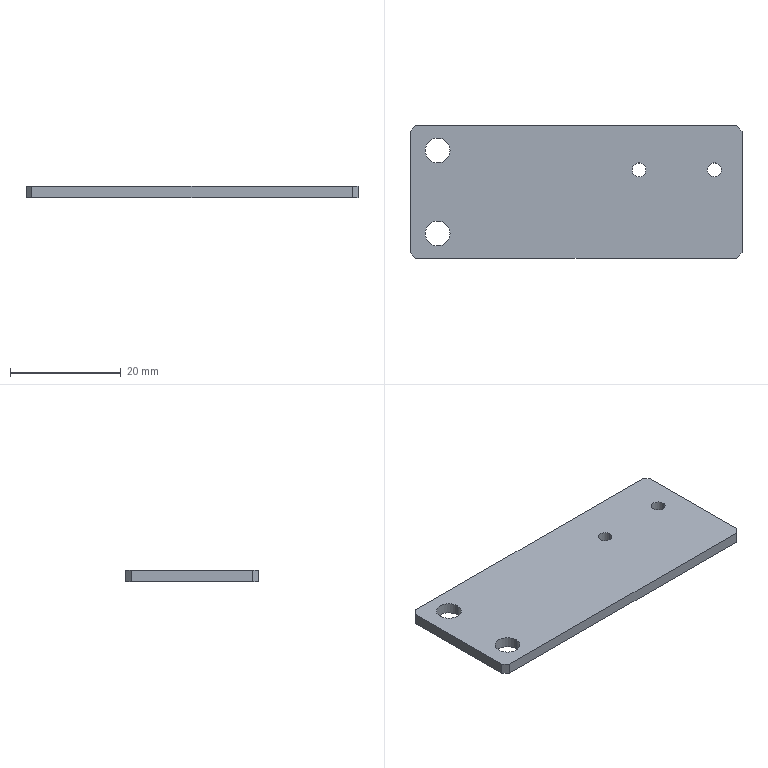Part | SolidWorks | features HoleWzd 2, Chamfer 1, FlatPattern 1, SMBaseFlange 1, SheetMetal 1 | 1 solid | 18 faces | box 60 x 24 x 2 mm | volume 2793 mm3 | plane 10 | cylinder 8 | commonest cylinder face diameters 2.5 x4 4.5 x4
STEP:
#1=CARTESIAN_POINT('',(10.15,4.,-2.));
#2=VERTEX_POINT('',#1);
#3=CARTESIAN_POINT('',(12.65,4.,-2.));
#4=VERTEX_POINT('',#3);
#5=CARTESIAN_POINT('',(11.4,4.,-2.));
#6=DIRECTION('',(0.,0.,1.));
#7=DIRECTION('',(1.,0.,0.));
#8=AXIS2_PLACEMENT_3D('',#5,#6,#7);
#9=CIRCLE('',#8,1.25);
#10=EDGE_CURVE('',#2,#4,#9,.T.);
#11=ORIENTED_EDGE('',*,*,#10,.F.);
#12=CARTESIAN_POINT('',(10.15,4.,0.));
#13=VERTEX_POINT('',#12);
#14=CARTESIAN_POINT('',(10.15,4.,0.));
#15=DIRECTION('',(0.,0.,1.));
#16=VECTOR('',#15,1000.);
#17=LINE('',#14,#16);
#18=EDGE_CURVE('',#2,#13,#17,.T.);
#19=ORIENTED_EDGE('',*,*,#18,.T.);
#20=CARTESIAN_POINT('',(12.65,4.,0.));
#21=VERTEX_POINT('',#20);
#22=CARTESIAN_POINT('',(11.4,4.,0.));
#23=DIRECTION('',(0.,0.,1.));
#24=DIRECTION('',(1.,0.,0.));
#25=AXIS2_PLACEMENT_3D('',#22,#23,#24);
#26=CIRCLE('',#25,1.25);
#27=EDGE_CURVE('',#13,#21,#26,.T.);
#28=ORIENTED_EDGE('',*,*,#27,.T.);
#29=CARTESIAN_POINT('',(12.65,4.,0.));
#30=DIRECTION('',(0.,0.,1.));
#31=VECTOR('',#30,1000.);
#32=LINE('',#29,#31);
#33=EDGE_CURVE('',#4,#21,#32,.T.);
#34=ORIENTED_EDGE('',*,*,#33,.F.);
#35=EDGE_LOOP('',(#11,#19,#28,#34));
#36=FACE_OUTER_BOUND('',#35,.T.);
#37=CARTESIAN_POINT('',(11.4,4.,0.));
#38=DIRECTION('',(0.,0.,1.));
#39=DIRECTION('',(1.,0.,0.));
#40=AXIS2_PLACEMENT_3D('',#37,#38,#39);
#41=CYLINDRICAL_SURFACE('',#40,1.25);
#42=ADVANCED_FACE('',(#36),#41,.F.);
#43=CARTESIAN_POINT('',(23.75,4.,-2.));
#44=VERTEX_POINT('',#43);
#45=CARTESIAN_POINT('',(26.25,4.,-2.));
#46=VERTEX_POINT('',#45);
#47=CARTESIAN_POINT('',(25.,4.,-2.));
#48=DIRECTION('',(0.,0.,1.));
#49=DIRECTION('',(1.,0.,0.));
#50=AXIS2_PLACEMENT_3D('',#47,#48,#49);
#51=CIRCLE('',#50,1.25);
#52=EDGE_CURVE('',#44,#46,#51,.T.);
#53=ORIENTED_EDGE('',*,*,#52,.F.);
#54=CARTESIAN_POINT('',(23.75,4.,0.));
#55=VERTEX_POINT('',#54);
#56=CARTESIAN_POINT('',(23.75,4.,0.));
#57=DIRECTION('',(0.,0.,1.));
#58=VECTOR('',#57,1000.);
#59=LINE('',#56,#58);
#60=EDGE_CURVE('',#44,#55,#59,.T.);
#61=ORIENTED_EDGE('',*,*,#60,.T.);
#62=CARTESIAN_POINT('',(26.25,4.,0.));
#63=VERTEX_POINT('',#62);
#64=CARTESIAN_POINT('',(25.,4.,0.));
#65=DIRECTION('',(0.,0.,1.));
#66=DIRECTION('',(1.,0.,0.));
#67=AXIS2_PLACEMENT_3D('',#64,#65,#66);
#68=CIRCLE('',#67,1.25);
#69=EDGE_CURVE('',#55,#63,#68,.T.);
#70=ORIENTED_EDGE('',*,*,#69,.T.);
#71=CARTESIAN_POINT('',(26.25,4.,0.));
#72=DIRECTION('',(0.,0.,1.));
#73=VECTOR('',#72,1000.);
#74=LINE('',#71,#73);
#75=EDGE_CURVE('',#46,#63,#74,.T.);
#76=ORIENTED_EDGE('',*,*,#75,.F.);
#77=EDGE_LOOP('',(#53,#61,#70,#76));
#78=FACE_OUTER_BOUND('',#77,.T.);
#79=CARTESIAN_POINT('',(25.,4.,0.));
#80=DIRECTION('',(0.,0.,1.));
#81=DIRECTION('',(1.,0.,0.));
#82=AXIS2_PLACEMENT_3D('',#79,#80,#81);
#83=CYLINDRICAL_SURFACE('',#82,1.25);
#84=ADVANCED_FACE('',(#78),#83,.F.);
#85=CARTESIAN_POINT('',(-27.25,7.5,-2.));
#86=VERTEX_POINT('',#85);
#87=CARTESIAN_POINT('',(-22.75,7.5,-2.));
#88=VERTEX_POINT('',#87);
#89=CARTESIAN_POINT('',(-25.,7.5,-2.));
#90=DIRECTION('',(0.,0.,1.));
#91=DIRECTION('',(1.,0.,0.));
#92=AXIS2_PLACEMENT_3D('',#89,#90,#91);
#93=CIRCLE('',#92,2.25);
#94=EDGE_CURVE('',#86,#88,#93,.T.);
#95=ORIENTED_EDGE('',*,*,#94,.F.);
#96=CARTESIAN_POINT('',(-27.25,7.5,0.));
#97=VERTEX_POINT('',#96);
#98=CARTESIAN_POINT('',(-27.25,7.5,0.));
#99=DIRECTION('',(0.,0.,1.));
#100=VECTOR('',#99,1000.);
#101=LINE('',#98,#100);
#102=EDGE_CURVE('',#86,#97,#101,.T.);
#103=ORIENTED_EDGE('',*,*,#102,.T.);
#104=CARTESIAN_POINT('',(-22.75,7.5,0.));
#105=VERTEX_POINT('',#104);
#106=CARTESIAN_POINT('',(-25.,7.5,0.));
#107=DIRECTION('',(0.,0.,1.));
#108=DIRECTION('',(1.,0.,0.));
#109=AXIS2_PLACEMENT_3D('',#106,#107,#108);
#110=CIRCLE('',#109,2.25);
#111=EDGE_CURVE('',#97,#105,#110,.T.);
#112=ORIENTED_EDGE('',*,*,#111,.T.);
#113=CARTESIAN_POINT('',(-22.75,7.5,0.));
#114=DIRECTION('',(0.,0.,1.));
#115=VECTOR('',#114,1000.);
#116=LINE('',#113,#115);
#117=EDGE_CURVE('',#88,#105,#116,.T.);
#118=ORIENTED_EDGE('',*,*,#117,.F.);
#119=EDGE_LOOP('',(#95,#103,#112,#118));
#120=FACE_OUTER_BOUND('',#119,.T.);
#121=CARTESIAN_POINT('',(-25.,7.5,0.));
#122=DIRECTION('',(0.,0.,1.));
#123=DIRECTION('',(1.,0.,0.));
#124=AXIS2_PLACEMENT_3D('',#121,#122,#123);
#125=CYLINDRICAL_SURFACE('',#124,2.25);
#126=ADVANCED_FACE('',(#120),#125,.F.);
#127=CARTESIAN_POINT('',(-27.25,-7.5,-2.));
#128=VERTEX_POINT('',#127);
#129=CARTESIAN_POINT('',(-22.75,-7.5,-2.));
#130=VERTEX_POINT('',#129);
#131=CARTESIAN_POINT('',(-25.,-7.5,-2.));
#132=DIRECTION('',(0.,0.,1.));
#133=DIRECTION('',(1.,0.,0.));
#134=AXIS2_PLACEMENT_3D('',#131,#132,#133);
#135=CIRCLE('',#134,2.25);
#136=EDGE_CURVE('',#128,#130,#135,.T.);
#137=ORIENTED_EDGE('',*,*,#136,.F.);
#138=CARTESIAN_POINT('',(-27.25,-7.5,0.));
#139=VERTEX_POINT('',#138);
#140=CARTESIAN_POINT('',(-27.25,-7.5,0.));
#141=DIRECTION('',(0.,0.,1.));
#142=VECTOR('',#141,1000.);
#143=LINE('',#140,#142);
#144=EDGE_CURVE('',#128,#139,#143,.T.);
#145=ORIENTED_EDGE('',*,*,#144,.T.);
#146=CARTESIAN_POINT('',(-22.75,-7.5,0.));
#147=VERTEX_POINT('',#146);
#148=CARTESIAN_POINT('',(-25.,-7.5,0.));
#149=DIRECTION('',(0.,0.,1.));
#150=DIRECTION('',(1.,0.,0.));
#151=AXIS2_PLACEMENT_3D('',#148,#149,#150);
#152=CIRCLE('',#151,2.25);
#153=EDGE_CURVE('',#139,#147,#152,.T.);
#154=ORIENTED_EDGE('',*,*,#153,.T.);
#155=CARTESIAN_POINT('',(-22.75,-7.5,0.));
#156=DIRECTION('',(0.,0.,1.));
#157=VECTOR('',#156,1000.);
#158=LINE('',#155,#157);
#159=EDGE_CURVE('',#130,#147,#158,.T.);
#160=ORIENTED_EDGE('',*,*,#159,.F.);
#161=EDGE_LOOP('',(#137,#145,#154,#160));
#162=FACE_OUTER_BOUND('',#161,.T.);
#163=CARTESIAN_POINT('',(-25.,-7.5,0.));
#164=DIRECTION('',(0.,0.,1.));
#165=DIRECTION('',(1.,0.,0.));
#166=AXIS2_PLACEMENT_3D('',#163,#164,#165);
#167=CYLINDRICAL_SURFACE('',#166,2.25);
#168=ADVANCED_FACE('',(#162),#167,.F.);
#169=CARTESIAN_POINT('',(30.,-11.,0.));
#170=VERTEX_POINT('',#169);
#171=CARTESIAN_POINT('',(30.,11.,0.));
#172=VERTEX_POINT('',#171);
#173=CARTESIAN_POINT('',(30.,12.,0.));
#174=DIRECTION('',(0.,1.,0.));
#175=VECTOR('',#174,1000.);
#176=LINE('',#173,#175);
#177=EDGE_CURVE('',#170,#172,#176,.T.);
#178=ORIENTED_EDGE('',*,*,#177,.F.);
#179=CARTESIAN_POINT('',(30.,-11.,-2.));
#180=VERTEX_POINT('',#179);
#181=CARTESIAN_POINT('',(30.,-11.,-2.));
#182=DIRECTION('',(0.,0.,-1.));
#183=VECTOR('',#182,1000.);
#184=LINE('',#181,#183);
#185=EDGE_CURVE('',#170,#180,#184,.T.);
#186=ORIENTED_EDGE('',*,*,#185,.T.);
#187=CARTESIAN_POINT('',(30.,11.,-2.));
#188=VERTEX_POINT('',#187);
#189=CARTESIAN_POINT('',(30.,12.,-2.));
#190=DIRECTION('',(0.,1.,0.));
#191=VECTOR('',#190,1000.);
#192=LINE('',#189,#191);
#193=EDGE_CURVE('',#180,#188,#192,.T.);
#194=ORIENTED_EDGE('',*,*,#193,.T.);
#195=CARTESIAN_POINT('',(30.,11.,-2.));
#196=DIRECTION('',(0.,0.,1.));
#197=VECTOR('',#196,1000.);
#198=LINE('',#195,#197);
#199=EDGE_CURVE('',#188,#172,#198,.T.);
#200=ORIENTED_EDGE('',*,*,#199,.T.);
#201=EDGE_LOOP('',(#178,#186,#194,#200));
#202=FACE_OUTER_BOUND('',#201,.T.);
#203=CARTESIAN_POINT('',(30.,12.,-2.));
#204=DIRECTION('',(1.,0.,0.));
#205=DIRECTION('',(0.,1.,0.));
#206=AXIS2_PLACEMENT_3D('',#203,#204,#205);
#207=PLANE('',#206);
#208=ADVANCED_FACE('',(#202),#207,.T.);
#209=CARTESIAN_POINT('',(-29.,-12.,0.));
#210=VERTEX_POINT('',#209);
#211=CARTESIAN_POINT('',(29.,-12.,0.));
#212=VERTEX_POINT('',#211);
#213=CARTESIAN_POINT('',(-30.,-12.,0.));
#214=DIRECTION('',(1.,0.,0.));
#215=VECTOR('',#214,1000.);
#216=LINE('',#213,#215);
#217=EDGE_CURVE('',#210,#212,#216,.T.);
#218=ORIENTED_EDGE('',*,*,#217,.F.);
#219=CARTESIAN_POINT('',(-29.,-12.,-2.));
#220=VERTEX_POINT('',#219);
#221=CARTESIAN_POINT('',(-29.,-12.,-2.));
#222=DIRECTION('',(0.,0.,-1.));
#223=VECTOR('',#222,1000.);
#224=LINE('',#221,#223);
#225=EDGE_CURVE('',#210,#220,#224,.T.);
#226=ORIENTED_EDGE('',*,*,#225,.T.);
#227=CARTESIAN_POINT('',(29.,-12.,-2.));
#228=VERTEX_POINT('',#227);
#229=CARTESIAN_POINT('',(-30.,-12.,-2.));
#230=DIRECTION('',(1.,0.,0.));
#231=VECTOR('',#230,1000.);
#232=LINE('',#229,#231);
#233=EDGE_CURVE('',#220,#228,#232,.T.);
#234=ORIENTED_EDGE('',*,*,#233,.T.);
#235=CARTESIAN_POINT('',(29.,-12.,-2.));
#236=DIRECTION('',(0.,0.,1.));
#237=VECTOR('',#236,1000.);
#238=LINE('',#235,#237);
#239=EDGE_CURVE('',#228,#212,#238,.T.);
#240=ORIENTED_EDGE('',*,*,#239,.T.);
#241=EDGE_LOOP('',(#218,#226,#234,#240));
#242=FACE_OUTER_BOUND('',#241,.T.);
#243=CARTESIAN_POINT('',(-30.,-12.,-2.));
#244=DIRECTION('',(0.,-1.,0.));
#245=DIRECTION('',(0.,0.,-1.));
#246=AXIS2_PLACEMENT_3D('',#243,#244,#245);
#247=PLANE('',#246);
#248=ADVANCED_FACE('',(#242),#247,.T.);
#249=CARTESIAN_POINT('',(-30.,11.,-2.));
#250=VERTEX_POINT('',#249);
#251=CARTESIAN_POINT('',(-30.,-11.,-2.));
#252=VERTEX_POINT('',#251);
#253=CARTESIAN_POINT('',(-30.,12.,-2.));
#254=DIRECTION('',(0.,-1.,0.));
#255=VECTOR('',#254,1000.);
#256=LINE('',#253,#255);
#257=EDGE_CURVE('',#250,#252,#256,.T.);
#258=ORIENTED_EDGE('',*,*,#257,.T.);
#259=CARTESIAN_POINT('',(-30.,-11.,0.));
#260=VERTEX_POINT('',#259);
#261=CARTESIAN_POINT('',(-30.,-11.,-2.));
#262=DIRECTION('',(0.,0.,1.));
#263=VECTOR('',#262,1000.);
#264=LINE('',#261,#263);
#265=EDGE_CURVE('',#252,#260,#264,.T.);
#266=ORIENTED_EDGE('',*,*,#265,.T.);
#267=CARTESIAN_POINT('',(-30.,11.,0.));
#268=VERTEX_POINT('',#267);
#269=CARTESIAN_POINT('',(-30.,12.,0.));
#270=DIRECTION('',(0.,-1.,0.));
#271=VECTOR('',#270,1000.);
#272=LINE('',#269,#271);
#273=EDGE_CURVE('',#268,#260,#272,.T.);
#274=ORIENTED_EDGE('',*,*,#273,.F.);
#275=CARTESIAN_POINT('',(-30.,11.,-2.));
#276=DIRECTION('',(0.,0.,-1.));
#277=VECTOR('',#276,1000.);
#278=LINE('',#275,#277);
#279=EDGE_CURVE('',#268,#250,#278,.T.);
#280=ORIENTED_EDGE('',*,*,#279,.T.);
#281=EDGE_LOOP('',(#258,#266,#274,#280));
#282=FACE_OUTER_BOUND('',#281,.T.);
#283=CARTESIAN_POINT('',(-30.,12.,-2.));
#284=DIRECTION('',(-1.,0.,0.));
#285=DIRECTION('',(0.,-1.,0.));
#286=AXIS2_PLACEMENT_3D('',#283,#284,#285);
#287=PLANE('',#286);
#288=ADVANCED_FACE('',(#282),#287,.T.);
#289=CARTESIAN_POINT('',(29.,12.,0.));
#290=VERTEX_POINT('',#289);
#291=CARTESIAN_POINT('',(-29.,12.,0.));
#292=VERTEX_POINT('',#291);
#293=CARTESIAN_POINT('',(-30.,12.,0.));
#294=DIRECTION('',(-1.,0.,0.));
#295=VECTOR('',#294,1000.);
#296=LINE('',#293,#295);
#297=EDGE_CURVE('',#290,#292,#296,.T.);
#298=ORIENTED_EDGE('',*,*,#297,.F.);
#299=CARTESIAN_POINT('',(29.,12.,-2.));
#300=VERTEX_POINT('',#299);
#301=CARTESIAN_POINT('',(29.,12.,-2.));
#302=DIRECTION('',(0.,0.,-1.));
#303=VECTOR('',#302,1000.);
#304=LINE('',#301,#303);
#305=EDGE_CURVE('',#290,#300,#304,.T.);
#306=ORIENTED_EDGE('',*,*,#305,.T.);
#307=CARTESIAN_POINT('',(-29.,12.,-2.));
#308=VERTEX_POINT('',#307);
#309=CARTESIAN_POINT('',(-30.,12.,-2.));
#310=DIRECTION('',(-1.,0.,0.));
#311=VECTOR('',#310,1000.);
#312=LINE('',#309,#311);
#313=EDGE_CURVE('',#300,#308,#312,.T.);
#314=ORIENTED_EDGE('',*,*,#313,.T.);
#315=CARTESIAN_POINT('',(-29.,12.,-2.));
#316=DIRECTION('',(0.,0.,1.));
#317=VECTOR('',#316,1000.);
#318=LINE('',#315,#317);
#319=EDGE_CURVE('',#308,#292,#318,.T.);
#320=ORIENTED_EDGE('',*,*,#319,.T.);
#321=EDGE_LOOP('',(#298,#306,#314,#320));
#322=FACE_OUTER_BOUND('',#321,.T.);
#323=CARTESIAN_POINT('',(-30.,12.,-2.));
#324=DIRECTION('',(0.,1.,0.));
#325=DIRECTION('',(0.,0.,1.));
#326=AXIS2_PLACEMENT_3D('',#323,#324,#325);
#327=PLANE('',#326);
#328=ADVANCED_FACE('',(#322),#327,.T.);
#329=CARTESIAN_POINT('',(11.4,4.,-2.));
#330=DIRECTION('',(0.,0.,1.));
#331=DIRECTION('',(1.,0.,0.));
#332=AXIS2_PLACEMENT_3D('',#329,#330,#331);
#333=CIRCLE('',#332,1.25);
#334=EDGE_CURVE('',#4,#2,#333,.T.);
#335=ORIENTED_EDGE('',*,*,#334,.T.);
#336=ORIENTED_EDGE('',*,*,#10,.T.);
#337=EDGE_LOOP('',(#335,#336));
#338=FACE_BOUND('',#337,.T.);
#339=CARTESIAN_POINT('',(25.,4.,-2.));
#340=DIRECTION('',(0.,0.,1.));
#341=DIRECTION('',(1.,0.,0.));
#342=AXIS2_PLACEMENT_3D('',#339,#340,#341);
#343=CIRCLE('',#342,1.25);
#344=EDGE_CURVE('',#46,#44,#343,.T.);
#345=ORIENTED_EDGE('',*,*,#344,.T.);
#346=ORIENTED_EDGE('',*,*,#52,.T.);
#347=EDGE_LOOP('',(#345,#346));
#348=FACE_BOUND('',#347,.T.);
#349=CARTESIAN_POINT('',(-25.,7.5,-2.));
#350=DIRECTION('',(0.,0.,1.));
#351=DIRECTION('',(1.,0.,0.));
#352=AXIS2_PLACEMENT_3D('',#349,#350,#351);
#353=CIRCLE('',#352,2.25);
#354=EDGE_CURVE('',#88,#86,#353,.T.);
#355=ORIENTED_EDGE('',*,*,#354,.T.);
#356=ORIENTED_EDGE('',*,*,#94,.T.);
#357=EDGE_LOOP('',(#355,#356));
#358=FACE_BOUND('',#357,.T.);
#359=CARTESIAN_POINT('',(-25.,-7.5,-2.));
#360=DIRECTION('',(0.,0.,1.));
#361=DIRECTION('',(1.,0.,0.));
#362=AXIS2_PLACEMENT_3D('',#359,#360,#361);
#363=CIRCLE('',#362,2.25);
#364=EDGE_CURVE('',#130,#128,#363,.T.);
#365=ORIENTED_EDGE('',*,*,#364,.T.);
#366=ORIENTED_EDGE('',*,*,#136,.T.);
#367=EDGE_LOOP('',(#365,#366));
#368=FACE_BOUND('',#367,.T.);
#369=ORIENTED_EDGE('',*,*,#233,.F.);
#370=CARTESIAN_POINT('',(-30.,-11.,-2.));
#371=DIRECTION('',(-0.7071,0.7071,0.));
#372=VECTOR('',#371,1000.);
#373=LINE('',#370,#372);
#374=EDGE_CURVE('',#220,#252,#373,.T.);
#375=ORIENTED_EDGE('',*,*,#374,.T.);
#376=ORIENTED_EDGE('',*,*,#257,.F.);
#377=CARTESIAN_POINT('',(-29.,12.,-2.));
#378=DIRECTION('',(0.7071,0.7071,0.));
#379=VECTOR('',#378,1000.);
#380=LINE('',#377,#379);
#381=EDGE_CURVE('',#250,#308,#380,.T.);
#382=ORIENTED_EDGE('',*,*,#381,.T.);
#383=ORIENTED_EDGE('',*,*,#313,.F.);
#384=CARTESIAN_POINT('',(30.,11.,-2.));
#385=DIRECTION('',(0.7071,-0.7071,0.));
#386=VECTOR('',#385,1000.);
#387=LINE('',#384,#386);
#388=EDGE_CURVE('',#300,#188,#387,.T.);
#389=ORIENTED_EDGE('',*,*,#388,.T.);
#390=ORIENTED_EDGE('',*,*,#193,.F.);
#391=CARTESIAN_POINT('',(29.,-12.,-2.));
#392=DIRECTION('',(-0.7071,-0.7071,0.));
#393=VECTOR('',#392,1000.);
#394=LINE('',#391,#393);
#395=EDGE_CURVE('',#180,#228,#394,.T.);
#396=ORIENTED_EDGE('',*,*,#395,.T.);
#397=EDGE_LOOP('',(#369,#375,#376,#382,#383,#389,#390,#396));
#398=FACE_OUTER_BOUND('',#397,.T.);
#399=CARTESIAN_POINT('',(0.,0.,-2.));
#400=DIRECTION('',(0.,0.,1.));
#401=DIRECTION('',(1.,0.,0.));
#402=AXIS2_PLACEMENT_3D('',#399,#400,#401);
#403=PLANE('',#402);
#404=ADVANCED_FACE('',(#338,#348,#358,#368,#398),#403,.F.);
#405=CARTESIAN_POINT('',(11.4,4.,0.));
#406=DIRECTION('',(0.,0.,1.));
#407=DIRECTION('',(1.,0.,0.));
#408=AXIS2_PLACEMENT_3D('',#405,#406,#407);
#409=CIRCLE('',#408,1.25);
#410=EDGE_CURVE('',#21,#13,#409,.T.);
#411=ORIENTED_EDGE('',*,*,#410,.F.);
#412=ORIENTED_EDGE('',*,*,#27,.F.);
#413=EDGE_LOOP('',(#411,#412));
#414=FACE_BOUND('',#413,.T.);
#415=CARTESIAN_POINT('',(25.,4.,0.));
#416=DIRECTION('',(0.,0.,1.));
#417=DIRECTION('',(1.,0.,0.));
#418=AXIS2_PLACEMENT_3D('',#415,#416,#417);
#419=CIRCLE('',#418,1.25);
#420=EDGE_CURVE('',#63,#55,#419,.T.);
#421=ORIENTED_EDGE('',*,*,#420,.F.);
#422=ORIENTED_EDGE('',*,*,#69,.F.);
#423=EDGE_LOOP('',(#421,#422));
#424=FACE_BOUND('',#423,.T.);
#425=CARTESIAN_POINT('',(-25.,7.5,0.));
#426=DIRECTION('',(0.,0.,1.));
#427=DIRECTION('',(1.,0.,0.));
#428=AXIS2_PLACEMENT_3D('',#425,#426,#427);
#429=CIRCLE('',#428,2.25);
#430=EDGE_CURVE('',#105,#97,#429,.T.);
#431=ORIENTED_EDGE('',*,*,#430,.F.);
#432=ORIENTED_EDGE('',*,*,#111,.F.);
#433=EDGE_LOOP('',(#431,#432));
#434=FACE_BOUND('',#433,.T.);
#435=CARTESIAN_POINT('',(-25.,-7.5,0.));
#436=DIRECTION('',(0.,0.,1.));
#437=DIRECTION('',(1.,0.,0.));
#438=AXIS2_PLACEMENT_3D('',#435,#436,#437);
#439=CIRCLE('',#438,2.25);
#440=EDGE_CURVE('',#147,#139,#439,.T.);
#441=ORIENTED_EDGE('',*,*,#440,.F.);
#442=ORIENTED_EDGE('',*,*,#153,.F.);
#443=EDGE_LOOP('',(#441,#442));
#444=FACE_BOUND('',#443,.T.);
#445=ORIENTED_EDGE('',*,*,#273,.T.);
#446=CARTESIAN_POINT('',(-20.5,-20.5,0.));
#447=DIRECTION('',(0.7071,-0.7071,0.));
#448=VECTOR('',#447,1000.);
#449=LINE('',#446,#448);
#450=EDGE_CURVE('',#260,#210,#449,.T.);
#451=ORIENTED_EDGE('',*,*,#450,.T.);
#452=ORIENTED_EDGE('',*,*,#217,.T.);
#453=CARTESIAN_POINT('',(20.5,-20.5,0.));
#454=DIRECTION('',(0.7071,0.7071,0.));
#455=VECTOR('',#454,1000.);
#456=LINE('',#453,#455);
#457=EDGE_CURVE('',#212,#170,#456,.T.);
#458=ORIENTED_EDGE('',*,*,#457,.T.);
#459=ORIENTED_EDGE('',*,*,#177,.T.);
#460=CARTESIAN_POINT('',(20.5,20.5,0.));
#461=DIRECTION('',(-0.7071,0.7071,0.));
#462=VECTOR('',#461,1000.);
#463=LINE('',#460,#462);
#464=EDGE_CURVE('',#172,#290,#463,.T.);
#465=ORIENTED_EDGE('',*,*,#464,.T.);
#466=ORIENTED_EDGE('',*,*,#297,.T.);
#467=CARTESIAN_POINT('',(-20.5,20.5,0.));
#468=DIRECTION('',(-0.7071,-0.7071,0.));
#469=VECTOR('',#468,1000.);
#470=LINE('',#467,#469);
#471=EDGE_CURVE('',#292,#268,#470,.T.);
#472=ORIENTED_EDGE('',*,*,#471,.T.);
#473=EDGE_LOOP('',(#445,#451,#452,#458,#459,#465,#466,#472));
#474=FACE_OUTER_BOUND('',#473,.T.);
#475=CARTESIAN_POINT('',(0.,0.,0.));
#476=DIRECTION('',(0.,0.,1.));
#477=DIRECTION('',(1.,0.,0.));
#478=AXIS2_PLACEMENT_3D('',#475,#476,#477);
#479=PLANE('',#478);
#480=ADVANCED_FACE('',(#414,#424,#434,#444,#474),#479,.T.);
#481=ORIENTED_EDGE('',*,*,#374,.F.);
#482=ORIENTED_EDGE('',*,*,#225,.F.);
#483=ORIENTED_EDGE('',*,*,#450,.F.);
#484=ORIENTED_EDGE('',*,*,#265,.F.);
#485=EDGE_LOOP('',(#481,#482,#483,#484));
#486=FACE_OUTER_BOUND('',#485,.T.);
#487=CARTESIAN_POINT('',(-30.,-11.,-2.));
#488=DIRECTION('',(0.7071,0.7071,0.));
#489=DIRECTION('',(0.,0.,1.));
#490=AXIS2_PLACEMENT_3D('',#487,#488,#489);
#491=PLANE('',#490);
#492=ADVANCED_FACE('',(#486),#491,.F.);
#493=ORIENTED_EDGE('',*,*,#395,.F.);
#494=ORIENTED_EDGE('',*,*,#185,.F.);
#495=ORIENTED_EDGE('',*,*,#457,.F.);
#496=ORIENTED_EDGE('',*,*,#239,.F.);
#497=EDGE_LOOP('',(#493,#494,#495,#496));
#498=FACE_OUTER_BOUND('',#497,.T.);
#499=CARTESIAN_POINT('',(29.,-12.,-2.));
#500=DIRECTION('',(-0.7071,0.7071,0.));
#501=DIRECTION('',(0.,0.,1.));
#502=AXIS2_PLACEMENT_3D('',#499,#500,#501);
#503=PLANE('',#502);
#504=ADVANCED_FACE('',(#498),#503,.F.);
#505=ORIENTED_EDGE('',*,*,#388,.F.);
#506=ORIENTED_EDGE('',*,*,#305,.F.);
#507=ORIENTED_EDGE('',*,*,#464,.F.);
#508=ORIENTED_EDGE('',*,*,#199,.F.);
#509=EDGE_LOOP('',(#505,#506,#507,#508));
#510=FACE_OUTER_BOUND('',#509,.T.);
#511=CARTESIAN_POINT('',(30.,11.,-2.));
#512=DIRECTION('',(-0.7071,-0.7071,0.));
#513=DIRECTION('',(0.,0.,1.));
#514=AXIS2_PLACEMENT_3D('',#511,#512,#513);
#515=PLANE('',#514);
#516=ADVANCED_FACE('',(#510),#515,.F.);
#517=ORIENTED_EDGE('',*,*,#381,.F.);
#518=ORIENTED_EDGE('',*,*,#279,.F.);
#519=ORIENTED_EDGE('',*,*,#471,.F.);
#520=ORIENTED_EDGE('',*,*,#319,.F.);
#521=EDGE_LOOP('',(#517,#518,#519,#520));
#522=FACE_OUTER_BOUND('',#521,.T.);
#523=CARTESIAN_POINT('',(-29.,12.,-2.));
#524=DIRECTION('',(0.7071,-0.7071,0.));
#525=DIRECTION('',(0.,0.,1.));
#526=AXIS2_PLACEMENT_3D('',#523,#524,#525);
#527=PLANE('',#526);
#528=ADVANCED_FACE('',(#522),#527,.F.);
#529=ORIENTED_EDGE('',*,*,#144,.F.);
#530=ORIENTED_EDGE('',*,*,#364,.F.);
#531=ORIENTED_EDGE('',*,*,#159,.T.);
#532=ORIENTED_EDGE('',*,*,#440,.T.);
#533=EDGE_LOOP('',(#529,#530,#531,#532));
#534=FACE_OUTER_BOUND('',#533,.T.);
#535=CARTESIAN_POINT('',(-25.,-7.5,0.));
#536=DIRECTION('',(0.,0.,1.));
#537=DIRECTION('',(1.,0.,0.));
#538=AXIS2_PLACEMENT_3D('',#535,#536,#537);
#539=CYLINDRICAL_SURFACE('',#538,2.25);
#540=ADVANCED_FACE('',(#534),#539,.F.);
#541=ORIENTED_EDGE('',*,*,#102,.F.);
#542=ORIENTED_EDGE('',*,*,#354,.F.);
#543=ORIENTED_EDGE('',*,*,#117,.T.);
#544=ORIENTED_EDGE('',*,*,#430,.T.);
#545=EDGE_LOOP('',(#541,#542,#543,#544));
#546=FACE_OUTER_BOUND('',#545,.T.);
#547=CARTESIAN_POINT('',(-25.,7.5,0.));
#548=DIRECTION('',(0.,0.,1.));
#549=DIRECTION('',(1.,0.,0.));
#550=AXIS2_PLACEMENT_3D('',#547,#548,#549);
#551=CYLINDRICAL_SURFACE('',#550,2.25);
#552=ADVANCED_FACE('',(#546),#551,.F.);
#553=ORIENTED_EDGE('',*,*,#60,.F.);
#554=ORIENTED_EDGE('',*,*,#344,.F.);
#555=ORIENTED_EDGE('',*,*,#75,.T.);
#556=ORIENTED_EDGE('',*,*,#420,.T.);
#557=EDGE_LOOP('',(#553,#554,#555,#556));
#558=FACE_OUTER_BOUND('',#557,.T.);
#559=CARTESIAN_POINT('',(25.,4.,0.));
#560=DIRECTION('',(0.,0.,1.));
#561=DIRECTION('',(1.,0.,0.));
#562=AXIS2_PLACEMENT_3D('',#559,#560,#561);
#563=CYLINDRICAL_SURFACE('',#562,1.25);
#564=ADVANCED_FACE('',(#558),#563,.F.);
#565=ORIENTED_EDGE('',*,*,#18,.F.);
#566=ORIENTED_EDGE('',*,*,#334,.F.);
#567=ORIENTED_EDGE('',*,*,#33,.T.);
#568=ORIENTED_EDGE('',*,*,#410,.T.);
#569=EDGE_LOOP('',(#565,#566,#567,#568));
#570=FACE_OUTER_BOUND('',#569,.T.);
#571=CARTESIAN_POINT('',(11.4,4.,0.));
#572=DIRECTION('',(0.,0.,1.));
#573=DIRECTION('',(1.,0.,0.));
#574=AXIS2_PLACEMENT_3D('',#571,#572,#573);
#575=CYLINDRICAL_SURFACE('',#574,1.25);
#576=ADVANCED_FACE('',(#570),#575,.F.);
#577=CLOSED_SHELL('',(#42,#84,#126,#168,#208,#248,#288,#328,#404,#480,#492,#504,#516,#528,#540,#552,#564,#576));
#578=MANIFOLD_SOLID_BREP('',#577);
#579=CARTESIAN_POINT('',(0.,0.,0.));
#580=DIRECTION('',(0.,0.,1.));
#581=DIRECTION('',(1.,0.,0.));
#582=AXIS2_PLACEMENT_3D('',#579,#580,#581);
#583=(LENGTH_UNIT()NAMED_UNIT(*)SI_UNIT(.MILLI.,.METRE.));
#584=UNCERTAINTY_MEASURE_WITH_UNIT(LENGTH_MEASURE(0.00001),#583,'','');
#585=(NAMED_UNIT(*)PLANE_ANGLE_UNIT()SI_UNIT($,.RADIAN.));
#586=(NAMED_UNIT(*)SI_UNIT($,.STERADIAN.)SOLID_ANGLE_UNIT());
#587=(GEOMETRIC_REPRESENTATION_CONTEXT(3)GLOBAL_UNCERTAINTY_ASSIGNED_CONTEXT((#584))GLOBAL_UNIT_ASSIGNED_CONTEXT((#583,#585,#586))REPRESENTATION_CONTEXT('',''));
#588=ADVANCED_BREP_SHAPE_REPRESENTATION('',(#578,#582),#587);